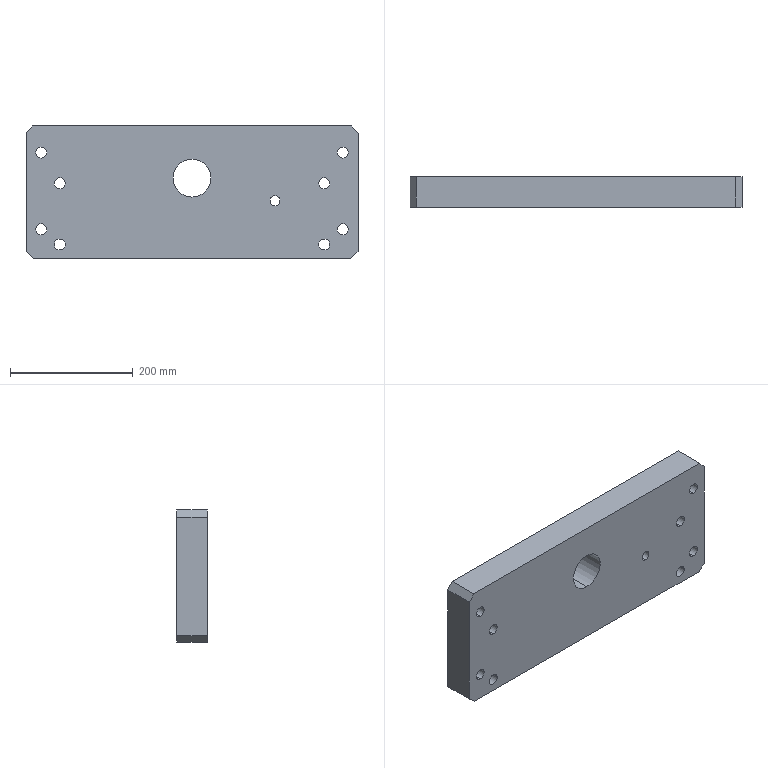Part | SolidWorks | features BaseBody 1 | 1 solid | 84 faces | box 542.001 x 50 x 215.5 mm | volume 5485358 mm3 | cylinder 44 | plane 32 | cone 8 | commonest cylinder face diameters 18 x16 26 x16 17.5 x8 16 x2 62 x2